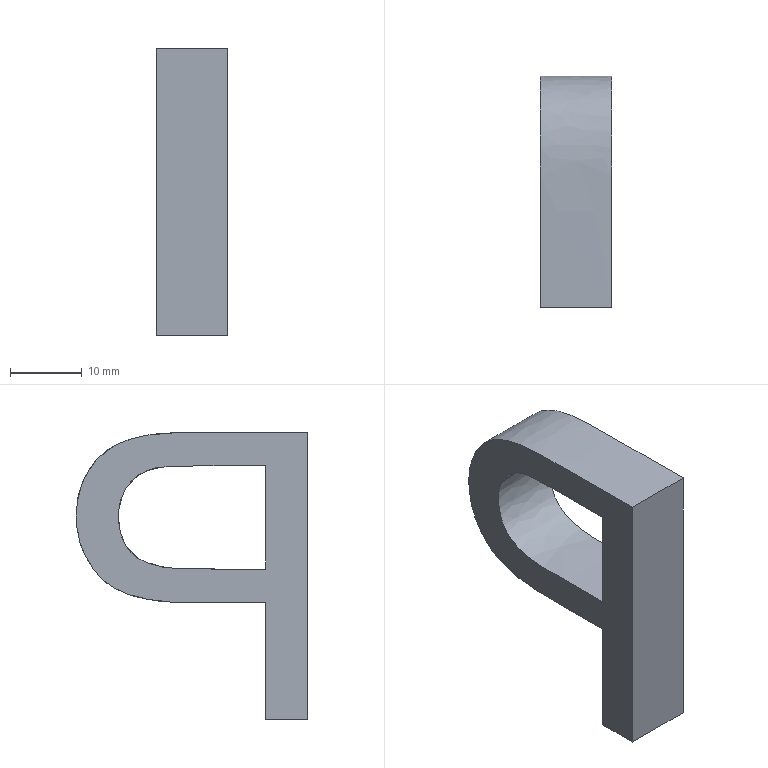Part | NX | features solid 2 | 1 solid | 8 faces | box 10 x 32.199 x 40 mm | volume 5391 mm3 | plane 6 | spline 2
STEP:
#1=CARTESIAN_POINT('',(2250.,-473.557,-634.665));
#2=VERTEX_POINT('',#1);
#3=CARTESIAN_POINT('',(2250.,-473.557,-649.029));
#4=VERTEX_POINT('',#3);
#5=CARTESIAN_POINT('',(2250.,-473.557,-634.665));
#6=CARTESIAN_POINT('',(2250.,-473.557,-639.453));
#7=CARTESIAN_POINT('',(2250.,-473.557,-644.241));
#8=CARTESIAN_POINT('',(2250.,-473.557,-649.029));
#9=B_SPLINE_CURVE_WITH_KNOTS('',3,(#5,#6,#7,#8),.UNSPECIFIED.,.F.,.F.,(4,4),(0.,0.1858),.PIECEWISE_BEZIER_KNOTS.);
#10=EDGE_CURVE('',#2,#4,#9,.T.);
#11=ORIENTED_EDGE('',*,*,#10,.F.);
#12=CARTESIAN_POINT('',(2260.,-473.557,-634.665));
#13=VERTEX_POINT('',#12);
#14=CARTESIAN_POINT('',(2260.,-473.557,-634.665));
#15=DIRECTION('',(-1.,0.,0.));
#16=VECTOR('',#15,1000.);
#17=LINE('',#14,#16);
#18=EDGE_CURVE('',#2,#13,#17,.F.);
#19=ORIENTED_EDGE('',*,*,#18,.T.);
#20=CARTESIAN_POINT('',(2260.,-473.557,-649.029));
#21=VERTEX_POINT('',#20);
#22=CARTESIAN_POINT('',(2260.,-473.557,-634.665));
#23=CARTESIAN_POINT('',(2260.,-473.557,-639.453));
#24=CARTESIAN_POINT('',(2260.,-473.557,-644.241));
#25=CARTESIAN_POINT('',(2260.,-473.557,-649.029));
#26=B_SPLINE_CURVE_WITH_KNOTS('',3,(#22,#23,#24,#25),.UNSPECIFIED.,.F.,.F.,(4,4),(0.,0.1858),.PIECEWISE_BEZIER_KNOTS.);
#27=EDGE_CURVE('',#13,#21,#26,.T.);
#28=ORIENTED_EDGE('',*,*,#27,.T.);
#29=CARTESIAN_POINT('',(2260.,-473.557,-649.029));
#30=DIRECTION('',(-1.,0.,0.));
#31=VECTOR('',#30,1000.);
#32=LINE('',#29,#31);
#33=EDGE_CURVE('',#21,#4,#32,.T.);
#34=ORIENTED_EDGE('',*,*,#33,.T.);
#35=EDGE_LOOP('',(#11,#19,#28,#34));
#36=FACE_BOUND('',#35,.T.);
#37=CARTESIAN_POINT('',(2260.,-473.557,-634.665));
#38=DIRECTION('',(0.,1.,0.));
#39=DIRECTION('',(-1.,0.,0.));
#40=AXIS2_PLACEMENT_3D('',#37,#38,#39);
#41=PLANE('',#40);
#42=ADVANCED_FACE('',(#36),#41,.T.);
#43=CARTESIAN_POINT('',(2250.,-473.557,-670.));
#44=VERTEX_POINT('',#43);
#45=CARTESIAN_POINT('',(2250.,-479.4,-670.));
#46=VERTEX_POINT('',#45);
#47=CARTESIAN_POINT('',(2250.,-473.557,-670.));
#48=CARTESIAN_POINT('',(2250.,-475.505,-670.));
#49=CARTESIAN_POINT('',(2250.,-477.452,-670.));
#50=CARTESIAN_POINT('',(2250.,-479.4,-670.));
#51=B_SPLINE_CURVE_WITH_KNOTS('',3,(#47,#48,#49,#50),.UNSPECIFIED.,.F.,.F.,(4,4),(0.,0.04053),.PIECEWISE_BEZIER_KNOTS.);
#52=EDGE_CURVE('',#44,#46,#51,.T.);
#53=ORIENTED_EDGE('',*,*,#52,.F.);
#54=CARTESIAN_POINT('',(2260.,-473.557,-670.));
#55=VERTEX_POINT('',#54);
#56=CARTESIAN_POINT('',(2260.,-473.557,-670.));
#57=DIRECTION('',(-1.,0.,0.));
#58=VECTOR('',#57,1000.);
#59=LINE('',#56,#58);
#60=EDGE_CURVE('',#55,#44,#59,.T.);
#61=ORIENTED_EDGE('',*,*,#60,.F.);
#62=CARTESIAN_POINT('',(2260.,-479.4,-670.));
#63=VERTEX_POINT('',#62);
#64=CARTESIAN_POINT('',(2260.,-473.557,-670.));
#65=CARTESIAN_POINT('',(2260.,-475.505,-670.));
#66=CARTESIAN_POINT('',(2260.,-477.452,-670.));
#67=CARTESIAN_POINT('',(2260.,-479.4,-670.));
#68=B_SPLINE_CURVE_WITH_KNOTS('',3,(#64,#65,#66,#67),.UNSPECIFIED.,.F.,.F.,(4,4),(0.,0.04053),.PIECEWISE_BEZIER_KNOTS.);
#69=EDGE_CURVE('',#55,#63,#68,.T.);
#70=ORIENTED_EDGE('',*,*,#69,.T.);
#71=CARTESIAN_POINT('',(2260.,-479.4,-670.));
#72=DIRECTION('',(-1.,0.,0.));
#73=VECTOR('',#72,1000.);
#74=LINE('',#71,#73);
#75=EDGE_CURVE('',#63,#46,#74,.T.);
#76=ORIENTED_EDGE('',*,*,#75,.T.);
#77=EDGE_LOOP('',(#53,#61,#70,#76));
#78=FACE_BOUND('',#77,.T.);
#79=CARTESIAN_POINT('',(2260.,-473.557,-670.));
#80=DIRECTION('',(0.,0.,-1.));
#81=DIRECTION('',(-1.,0.,0.));
#82=AXIS2_PLACEMENT_3D('',#79,#80,#81);
#83=PLANE('',#82);
#84=ADVANCED_FACE('',(#78),#83,.T.);
#85=CARTESIAN_POINT('',(2250.,-479.4,-630.));
#86=VERTEX_POINT('',#85);
#87=CARTESIAN_POINT('',(2250.,-479.4,-670.));
#88=CARTESIAN_POINT('',(2250.,-479.4,-656.667));
#89=CARTESIAN_POINT('',(2250.,-479.4,-643.333));
#90=CARTESIAN_POINT('',(2250.,-479.4,-630.));
#91=B_SPLINE_CURVE_WITH_KNOTS('',3,(#87,#88,#89,#90),.UNSPECIFIED.,.F.,.F.,(4,4),(0.04053,0.3179),.PIECEWISE_BEZIER_KNOTS.);
#92=EDGE_CURVE('',#46,#86,#91,.T.);
#93=ORIENTED_EDGE('',*,*,#92,.F.);
#94=ORIENTED_EDGE('',*,*,#75,.F.);
#95=CARTESIAN_POINT('',(2260.,-479.4,-630.));
#96=VERTEX_POINT('',#95);
#97=CARTESIAN_POINT('',(2260.,-479.4,-670.));
#98=CARTESIAN_POINT('',(2260.,-479.4,-656.667));
#99=CARTESIAN_POINT('',(2260.,-479.4,-643.333));
#100=CARTESIAN_POINT('',(2260.,-479.4,-630.));
#101=B_SPLINE_CURVE_WITH_KNOTS('',3,(#97,#98,#99,#100),.UNSPECIFIED.,.F.,.F.,(4,4),(0.04053,0.3179),.PIECEWISE_BEZIER_KNOTS.);
#102=EDGE_CURVE('',#63,#96,#101,.T.);
#103=ORIENTED_EDGE('',*,*,#102,.T.);
#104=CARTESIAN_POINT('',(2260.,-479.4,-630.));
#105=DIRECTION('',(-1.,0.,0.));
#106=VECTOR('',#105,1000.);
#107=LINE('',#104,#106);
#108=EDGE_CURVE('',#96,#86,#107,.T.);
#109=ORIENTED_EDGE('',*,*,#108,.T.);
#110=EDGE_LOOP('',(#93,#94,#103,#109));
#111=FACE_BOUND('',#110,.T.);
#112=CARTESIAN_POINT('',(2260.,-479.4,-670.));
#113=DIRECTION('',(0.,-1.,0.));
#114=DIRECTION('',(1.,0.,0.));
#115=AXIS2_PLACEMENT_3D('',#112,#113,#114);
#116=PLANE('',#115);
#117=ADVANCED_FACE('',(#111),#116,.T.);
#118=CARTESIAN_POINT('',(2250.,-473.557,-653.694));
#119=VERTEX_POINT('',#118);
#120=CARTESIAN_POINT('',(2250.,-479.4,-630.));
#121=CARTESIAN_POINT('',(2250.,-474.102,-630.));
#122=CARTESIAN_POINT('',(2250.,-468.805,-630.));
#123=CARTESIAN_POINT('',(2250.,-463.507,-630.02));
#124=CARTESIAN_POINT('',(2250.,-460.693,-630.031));
#125=CARTESIAN_POINT('',(2250.,-458.551,-630.153));
#126=CARTESIAN_POINT('',(2250.,-454.989,-630.747));
#127=CARTESIAN_POINT('',(2250.,-453.259,-631.361));
#128=CARTESIAN_POINT('',(2250.,-450.437,-633.202));
#129=CARTESIAN_POINT('',(2250.,-449.312,-634.497));
#130=CARTESIAN_POINT('',(2250.,-448.468,-636.14));
#131=CARTESIAN_POINT('',(2250.,-447.614,-637.801));
#132=CARTESIAN_POINT('',(2250.,-447.201,-639.621));
#133=CARTESIAN_POINT('',(2250.,-447.201,-644.975));
#134=CARTESIAN_POINT('',(2250.,-448.318,-647.866));
#135=CARTESIAN_POINT('',(2250.,-450.581,-650.206));
#136=CARTESIAN_POINT('',(2250.,-452.846,-652.547));
#137=CARTESIAN_POINT('',(2250.,-456.945,-653.725));
#138=CARTESIAN_POINT('',(2250.,-466.429,-653.676));
#139=CARTESIAN_POINT('',(2250.,-469.993,-653.694));
#140=CARTESIAN_POINT('',(2250.,-473.557,-653.694));
#141=B_SPLINE_CURVE_WITH_KNOTS('',3,(#120,#121,#122,#123,#124,#125,#126,#127,#128,#129,#130,#131,#132,#133,#134,#135,#136,#137,#138,#139,#140),.UNSPECIFIED.,.F.,.F.,(4,3,2,2,3,2,3,2,4),(0.3179,0.4282,0.4729,0.5366,0.6006,0.6433,0.7184,0.8183,0.8785),.UNSPECIFIED.);
#142=EDGE_CURVE('',#86,#119,#141,.T.);
#143=ORIENTED_EDGE('',*,*,#142,.F.);
#144=ORIENTED_EDGE('',*,*,#108,.F.);
#145=CARTESIAN_POINT('',(2260.,-473.557,-653.694));
#146=VERTEX_POINT('',#145);
#147=CARTESIAN_POINT('',(2260.,-479.4,-630.));
#148=CARTESIAN_POINT('',(2260.,-474.102,-630.));
#149=CARTESIAN_POINT('',(2260.,-468.805,-630.));
#150=CARTESIAN_POINT('',(2260.,-463.507,-630.02));
#151=CARTESIAN_POINT('',(2260.,-460.693,-630.031));
#152=CARTESIAN_POINT('',(2260.,-458.551,-630.153));
#153=CARTESIAN_POINT('',(2260.,-454.989,-630.747));
#154=CARTESIAN_POINT('',(2260.,-453.259,-631.361));
#155=CARTESIAN_POINT('',(2260.,-450.437,-633.202));
#156=CARTESIAN_POINT('',(2260.,-449.312,-634.497));
#157=CARTESIAN_POINT('',(2260.,-448.468,-636.14));
#158=CARTESIAN_POINT('',(2260.,-447.614,-637.801));
#159=CARTESIAN_POINT('',(2260.,-447.201,-639.621));
#160=CARTESIAN_POINT('',(2260.,-447.201,-644.975));
#161=CARTESIAN_POINT('',(2260.,-448.318,-647.866));
#162=CARTESIAN_POINT('',(2260.,-450.581,-650.206));
#163=CARTESIAN_POINT('',(2260.,-452.846,-652.547));
#164=CARTESIAN_POINT('',(2260.,-456.945,-653.725));
#165=CARTESIAN_POINT('',(2260.,-466.429,-653.676));
#166=CARTESIAN_POINT('',(2260.,-469.993,-653.694));
#167=CARTESIAN_POINT('',(2260.,-473.557,-653.694));
#168=B_SPLINE_CURVE_WITH_KNOTS('',3,(#147,#148,#149,#150,#151,#152,#153,#154,#155,#156,#157,#158,#159,#160,#161,#162,#163,#164,#165,#166,#167),.UNSPECIFIED.,.F.,.F.,(4,3,2,2,3,2,3,2,4),(0.3179,0.4282,0.4729,0.5366,0.6006,0.6433,0.7184,0.8183,0.8785),.UNSPECIFIED.);
#169=EDGE_CURVE('',#96,#146,#168,.T.);
#170=ORIENTED_EDGE('',*,*,#169,.T.);
#171=CARTESIAN_POINT('',(2260.,-473.557,-653.694));
#172=DIRECTION('',(-1.,0.,0.));
#173=VECTOR('',#172,1000.);
#174=LINE('',#171,#173);
#175=EDGE_CURVE('',#146,#119,#174,.T.);
#176=ORIENTED_EDGE('',*,*,#175,.T.);
#177=EDGE_LOOP('',(#143,#144,#170,#176));
#178=FACE_BOUND('',#177,.T.);
#179=CARTESIAN_POINT('',(2260.,-479.4,-630.));
#180=CARTESIAN_POINT('',(2250.,-479.4,-630.));
#181=CARTESIAN_POINT('',(2260.,-477.716,-630.));
#182=CARTESIAN_POINT('',(2250.,-477.716,-630.));
#183=CARTESIAN_POINT('',(2260.,-474.347,-630.));
#184=CARTESIAN_POINT('',(2250.,-474.347,-630.));
#185=CARTESIAN_POINT('',(2260.,-470.142,-630.003));
#186=CARTESIAN_POINT('',(2250.,-470.142,-630.003));
#187=CARTESIAN_POINT('',(2260.,-467.188,-630.009));
#188=CARTESIAN_POINT('',(2250.,-467.188,-630.009));
#189=CARTESIAN_POINT('',(2260.,-465.516,-630.013));
#190=CARTESIAN_POINT('',(2250.,-465.516,-630.013));
#191=CARTESIAN_POINT('',(2260.,-464.432,-630.017));
#192=CARTESIAN_POINT('',(2250.,-464.432,-630.017));
#193=CARTESIAN_POINT('',(2260.,-463.656,-630.019));
#194=CARTESIAN_POINT('',(2250.,-463.656,-630.019));
#195=CARTESIAN_POINT('',(2260.,-462.547,-630.025));
#196=CARTESIAN_POINT('',(2250.,-462.547,-630.025));
#197=CARTESIAN_POINT('',(2260.,-460.797,-630.061));
#198=CARTESIAN_POINT('',(2250.,-460.797,-630.061));
#199=CARTESIAN_POINT('',(2260.,-458.64,-630.177));
#200=CARTESIAN_POINT('',(2250.,-458.64,-630.177));
#201=CARTESIAN_POINT('',(2260.,-456.768,-630.425));
#202=CARTESIAN_POINT('',(2250.,-456.768,-630.425));
#203=CARTESIAN_POINT('',(2260.,-454.638,-630.914));
#204=CARTESIAN_POINT('',(2250.,-454.638,-630.914));
#205=CARTESIAN_POINT('',(2260.,-452.784,-631.656));
#206=CARTESIAN_POINT('',(2250.,-452.784,-631.656));
#207=CARTESIAN_POINT('',(2260.,-451.243,-632.668));
#208=CARTESIAN_POINT('',(2250.,-451.243,-632.668));
#209=CARTESIAN_POINT('',(2260.,-450.215,-633.593));
#210=CARTESIAN_POINT('',(2250.,-450.215,-633.593));
#211=CARTESIAN_POINT('',(2260.,-449.461,-634.509));
#212=CARTESIAN_POINT('',(2250.,-449.461,-634.509));
#213=CARTESIAN_POINT('',(2260.,-448.932,-635.3));
#214=CARTESIAN_POINT('',(2250.,-448.932,-635.3));
#215=CARTESIAN_POINT('',(2260.,-448.636,-635.819));
#216=CARTESIAN_POINT('',(2250.,-448.636,-635.819));
#217=CARTESIAN_POINT('',(2260.,-448.485,-636.106));
#218=CARTESIAN_POINT('',(2250.,-448.485,-636.106));
#219=CARTESIAN_POINT('',(2260.,-448.301,-636.471));
#220=CARTESIAN_POINT('',(2250.,-448.301,-636.471));
#221=CARTESIAN_POINT('',(2260.,-448.034,-637.063));
#222=CARTESIAN_POINT('',(2250.,-448.034,-637.063));
#223=CARTESIAN_POINT('',(2260.,-447.574,-638.322));
#224=CARTESIAN_POINT('',(2250.,-447.574,-638.322));
#225=CARTESIAN_POINT('',(2260.,-447.2,-640.182));
#226=CARTESIAN_POINT('',(2250.,-447.2,-640.182));
#227=CARTESIAN_POINT('',(2260.,-447.173,-642.595));
#228=CARTESIAN_POINT('',(2250.,-447.173,-642.595));
#229=CARTESIAN_POINT('',(2260.,-447.512,-644.822));
#230=CARTESIAN_POINT('',(2250.,-447.512,-644.822));
#231=CARTESIAN_POINT('',(2260.,-448.216,-646.878));
#232=CARTESIAN_POINT('',(2250.,-448.216,-646.878));
#233=CARTESIAN_POINT('',(2260.,-449.12,-648.452));
#234=CARTESIAN_POINT('',(2250.,-449.12,-648.452));
#235=CARTESIAN_POINT('',(2260.,-449.899,-649.459));
#236=CARTESIAN_POINT('',(2250.,-449.899,-649.459));
#237=CARTESIAN_POINT('',(2260.,-450.418,-650.04));
#238=CARTESIAN_POINT('',(2250.,-450.418,-650.04));
#239=CARTESIAN_POINT('',(2260.,-450.865,-650.499));
#240=CARTESIAN_POINT('',(2250.,-450.865,-650.499));
#241=CARTESIAN_POINT('',(2260.,-451.392,-650.953));
#242=CARTESIAN_POINT('',(2250.,-451.392,-650.953));
#243=CARTESIAN_POINT('',(2260.,-452.396,-651.655));
#244=CARTESIAN_POINT('',(2250.,-452.396,-651.655));
#245=CARTESIAN_POINT('',(2260.,-453.845,-652.382));
#246=CARTESIAN_POINT('',(2250.,-453.845,-652.382));
#247=CARTESIAN_POINT('',(2260.,-456.626,-653.262));
#248=CARTESIAN_POINT('',(2250.,-456.626,-653.262));
#249=CARTESIAN_POINT('',(2260.,-460.057,-653.716));
#250=CARTESIAN_POINT('',(2250.,-460.057,-653.716));
#251=CARTESIAN_POINT('',(2260.,-464.22,-653.685));
#252=CARTESIAN_POINT('',(2250.,-464.22,-653.685));
#253=CARTESIAN_POINT('',(2260.,-468.367,-653.686));
#254=CARTESIAN_POINT('',(2250.,-468.367,-653.686));
#255=CARTESIAN_POINT('',(2260.,-471.482,-653.694));
#256=CARTESIAN_POINT('',(2250.,-471.482,-653.694));
#257=CARTESIAN_POINT('',(2260.,-473.557,-653.694));
#258=CARTESIAN_POINT('',(2250.,-473.557,-653.694));
#259=B_SPLINE_SURFACE_WITH_KNOTS('',3,1,((#179,#180),(#181,#182),(#183,#184),(#185,#186),(#187,#188),(#189,#190),(#191,#192),(#193,#194),(#195,#196),(#197,#198),(#199,#200),(#201,#202),(#203,#204),(#205,#206),(#207,#208),(#209,#210),(#211,#212),(#213,#214),(#215,#216),(#217,#218),(#219,#220),(#221,#222),(#223,#224),(#225,#226),(#227,#228),(#229,#230),(#231,#232),(#233,#234),(#235,#236),(#237,#238),(#239,#240),(#241,#242),(#243,#244),(#245,#246),(#247,#248),(#249,#250),(#251,#252),(#253,#254),(#255,#256),(#257,#258)),.SURF_OF_LINEAR_EXTRUSION.,.F.,.F.,.F.,(4,1,1,1,1,1,1,1,1,1,1,1,1,1,1,1,1,1,1,1,1,1,1,1,1,1,1,1,1,1,1,1,1,1,1,1,1,4),(2,2),(0.3179,0.353,0.388,0.4055,0.4143,0.423,0.4274,0.4318,0.4406,0.4581,0.4756,0.4931,0.5282,0.5457,0.5632,0.5807,0.5895,0.5982,0.6004,0.6026,0.607,0.6157,0.6333,0.6508,0.6683,0.6858,0.7033,0.7121,0.7165,0.7208,0.7296,0.7384,0.7559,0.7734,0.8084,0.8259,0.8435,0.8785),(0.,1.),.UNSPECIFIED.);
#260=ADVANCED_FACE('',(#178),#259,.T.);
#261=CARTESIAN_POINT('',(2250.,-473.557,-653.694));
#262=CARTESIAN_POINT('',(2250.,-473.557,-659.129));
#263=CARTESIAN_POINT('',(2250.,-473.557,-664.565));
#264=CARTESIAN_POINT('',(2250.,-473.557,-670.));
#265=B_SPLINE_CURVE_WITH_KNOTS('',3,(#261,#262,#263,#264),.UNSPECIFIED.,.F.,.F.,(4,4),(0.8785,1.),.PIECEWISE_BEZIER_KNOTS.);
#266=EDGE_CURVE('',#119,#44,#265,.T.);
#267=ORIENTED_EDGE('',*,*,#266,.F.);
#268=ORIENTED_EDGE('',*,*,#175,.F.);
#269=CARTESIAN_POINT('',(2260.,-473.557,-653.694));
#270=CARTESIAN_POINT('',(2260.,-473.557,-659.129));
#271=CARTESIAN_POINT('',(2260.,-473.557,-664.565));
#272=CARTESIAN_POINT('',(2260.,-473.557,-670.));
#273=B_SPLINE_CURVE_WITH_KNOTS('',3,(#269,#270,#271,#272),.UNSPECIFIED.,.F.,.F.,(4,4),(0.8785,1.),.PIECEWISE_BEZIER_KNOTS.);
#274=EDGE_CURVE('',#146,#55,#273,.T.);
#275=ORIENTED_EDGE('',*,*,#274,.T.);
#276=ORIENTED_EDGE('',*,*,#60,.T.);
#277=EDGE_LOOP('',(#267,#268,#275,#276));
#278=FACE_BOUND('',#277,.T.);
#279=CARTESIAN_POINT('',(2260.,-473.557,-653.694));
#280=DIRECTION('',(0.,1.,0.));
#281=DIRECTION('',(-1.,0.,0.));
#282=AXIS2_PLACEMENT_3D('',#279,#280,#281);
#283=PLANE('',#282);
#284=ADVANCED_FACE('',(#278),#283,.T.);
#285=CARTESIAN_POINT('',(2250.,-473.557,-649.029));
#286=CARTESIAN_POINT('',(2250.,-469.993,-649.029));
#287=CARTESIAN_POINT('',(2250.,-466.429,-649.029));
#288=CARTESIAN_POINT('',(2250.,-459.3,-649.029));
#289=CARTESIAN_POINT('',(2250.,-456.761,-648.432));
#290=CARTESIAN_POINT('',(2250.,-453.801,-645.869));
#291=CARTESIAN_POINT('',(2250.,-453.06,-644.057));
#292=CARTESIAN_POINT('',(2250.,-453.06,-640.08));
#293=CARTESIAN_POINT('',(2250.,-453.473,-638.642));
#294=CARTESIAN_POINT('',(2250.,-455.24,-636.236));
#295=CARTESIAN_POINT('',(2250.,-456.394,-635.446));
#296=CARTESIAN_POINT('',(2250.,-457.837,-635.052));
#297=CARTESIAN_POINT('',(2250.,-458.75,-634.803));
#298=CARTESIAN_POINT('',(2250.,-460.448,-634.681));
#299=CARTESIAN_POINT('',(2250.,-466.49,-634.644));
#300=CARTESIAN_POINT('',(2250.,-470.023,-634.665));
#301=CARTESIAN_POINT('',(2250.,-473.557,-634.665));
#302=B_SPLINE_CURVE_WITH_KNOTS('',3,(#285,#286,#287,#288,#289,#290,#291,#292,#293,#294,#295,#296,#297,#298,#299,#300,#301),.UNSPECIFIED.,.F.,.F.,(4,2,2,2,2,3,2,4),(0.1858,0.324,0.4623,0.5999,0.6976,0.7946,0.8799,1.),.UNSPECIFIED.);
#303=EDGE_CURVE('',#4,#2,#302,.T.);
#304=ORIENTED_EDGE('',*,*,#303,.F.);
#305=ORIENTED_EDGE('',*,*,#33,.F.);
#306=CARTESIAN_POINT('',(2260.,-473.557,-649.029));
#307=CARTESIAN_POINT('',(2260.,-469.993,-649.029));
#308=CARTESIAN_POINT('',(2260.,-466.429,-649.029));
#309=CARTESIAN_POINT('',(2260.,-459.3,-649.029));
#310=CARTESIAN_POINT('',(2260.,-456.761,-648.432));
#311=CARTESIAN_POINT('',(2260.,-453.801,-645.869));
#312=CARTESIAN_POINT('',(2260.,-453.06,-644.057));
#313=CARTESIAN_POINT('',(2260.,-453.06,-640.08));
#314=CARTESIAN_POINT('',(2260.,-453.473,-638.642));
#315=CARTESIAN_POINT('',(2260.,-455.24,-636.236));
#316=CARTESIAN_POINT('',(2260.,-456.394,-635.446));
#317=CARTESIAN_POINT('',(2260.,-457.837,-635.052));
#318=CARTESIAN_POINT('',(2260.,-458.75,-634.803));
#319=CARTESIAN_POINT('',(2260.,-460.448,-634.681));
#320=CARTESIAN_POINT('',(2260.,-466.49,-634.644));
#321=CARTESIAN_POINT('',(2260.,-470.023,-634.665));
#322=CARTESIAN_POINT('',(2260.,-473.557,-634.665));
#323=B_SPLINE_CURVE_WITH_KNOTS('',3,(#306,#307,#308,#309,#310,#311,#312,#313,#314,#315,#316,#317,#318,#319,#320,#321,#322),.UNSPECIFIED.,.F.,.F.,(4,2,2,2,2,3,2,4),(0.1858,0.324,0.4623,0.5999,0.6976,0.7946,0.8799,1.),.UNSPECIFIED.);
#324=EDGE_CURVE('',#21,#13,#323,.T.);
#325=ORIENTED_EDGE('',*,*,#324,.T.);
#326=ORIENTED_EDGE('',*,*,#18,.F.);
#327=EDGE_LOOP('',(#304,#305,#325,#326));
#328=FACE_BOUND('',#327,.T.);
#329=CARTESIAN_POINT('',(2260.,-473.557,-649.029));
#330=CARTESIAN_POINT('',(2250.,-473.557,-649.029));
#331=CARTESIAN_POINT('',(2260.,-470.933,-649.029));
#332=CARTESIAN_POINT('',(2250.,-470.933,-649.029));
#333=CARTESIAN_POINT('',(2260.,-467.653,-649.03));
#334=CARTESIAN_POINT('',(2250.,-467.653,-649.03));
#335=CARTESIAN_POINT('',(2260.,-463.72,-649.028));
#336=CARTESIAN_POINT('',(2250.,-463.72,-649.028));
#337=CARTESIAN_POINT('',(2260.,-461.089,-649.033));
#338=CARTESIAN_POINT('',(2250.,-461.089,-649.033));
#339=CARTESIAN_POINT('',(2260.,-458.368,-648.704));
#340=CARTESIAN_POINT('',(2250.,-458.368,-648.704));
#341=CARTESIAN_POINT('',(2260.,-455.925,-647.805));
#342=CARTESIAN_POINT('',(2250.,-455.925,-647.805));
#343=CARTESIAN_POINT('',(2260.,-454.352,-646.342));
#344=CARTESIAN_POINT('',(2250.,-454.352,-646.342));
#345=CARTESIAN_POINT('',(2260.,-453.351,-644.476));
#346=CARTESIAN_POINT('',(2250.,-453.351,-644.476));
#347=CARTESIAN_POINT('',(2260.,-452.963,-642.117));
#348=CARTESIAN_POINT('',(2250.,-452.963,-642.117));
#349=CARTESIAN_POINT('',(2260.,-453.189,-639.561));
#350=CARTESIAN_POINT('',(2250.,-453.189,-639.561));
#351=CARTESIAN_POINT('',(2260.,-454.169,-637.471));
#352=CARTESIAN_POINT('',(2250.,-454.169,-637.471));
#353=CARTESIAN_POINT('',(2260.,-455.539,-636.102));
#354=CARTESIAN_POINT('',(2250.,-455.539,-636.102));
#355=CARTESIAN_POINT('',(2260.,-456.797,-635.388));
#356=CARTESIAN_POINT('',(2250.,-456.797,-635.388));
#357=CARTESIAN_POINT('',(2260.,-457.77,-635.053));
#358=CARTESIAN_POINT('',(2250.,-457.77,-635.053));
#359=CARTESIAN_POINT('',(2260.,-458.347,-634.935));
#360=CARTESIAN_POINT('',(2250.,-458.347,-634.935));
#361=CARTESIAN_POINT('',(2260.,-459.137,-634.819));
#362=CARTESIAN_POINT('',(2250.,-459.137,-634.819));
#363=CARTESIAN_POINT('',(2260.,-460.361,-634.721));
#364=CARTESIAN_POINT('',(2250.,-460.361,-634.721));
#365=CARTESIAN_POINT('',(2260.,-462.283,-634.663));
#366=CARTESIAN_POINT('',(2250.,-462.283,-634.663));
#367=CARTESIAN_POINT('',(2260.,-465.35,-634.656));
#368=CARTESIAN_POINT('',(2250.,-465.35,-634.656));
#369=CARTESIAN_POINT('',(2260.,-469.056,-634.657));
#370=CARTESIAN_POINT('',(2250.,-469.056,-634.657));
#371=CARTESIAN_POINT('',(2260.,-472.06,-634.665));
#372=CARTESIAN_POINT('',(2250.,-472.06,-634.665));
#373=CARTESIAN_POINT('',(2260.,-473.557,-634.665));
#374=CARTESIAN_POINT('',(2250.,-473.557,-634.665));
#375=B_SPLINE_SURFACE_WITH_KNOTS('',3,1,((#329,#330),(#331,#332),(#333,#334),(#335,#336),(#337,#338),(#339,#340),(#341,#342),(#343,#344),(#345,#346),(#347,#348),(#349,#350),(#351,#352),(#353,#354),(#355,#356),(#357,#358),(#359,#360),(#361,#362),(#363,#364),(#365,#366),(#367,#368),(#369,#370),(#371,#372),(#373,#374)),.SURF_OF_LINEAR_EXTRUSION.,.F.,.F.,.F.,(4,1,1,1,1,1,1,1,1,1,1,1,1,1,1,1,1,1,1,1,4),(2,2),(0.1858,0.2875,0.313,0.3384,0.3893,0.4402,0.4911,0.542,0.5929,0.6438,0.6947,0.7455,0.771,0.7964,0.8092,0.8219,0.8473,0.8728,0.8982,0.9491,1.),(0.,1.),.UNSPECIFIED.);
#376=ADVANCED_FACE('',(#328),#375,.T.);
#377=ORIENTED_EDGE('',*,*,#69,.F.);
#378=ORIENTED_EDGE('',*,*,#274,.F.);
#379=ORIENTED_EDGE('',*,*,#169,.F.);
#380=ORIENTED_EDGE('',*,*,#102,.F.);
#381=EDGE_LOOP('',(#377,#378,#379,#380));
#382=FACE_BOUND('',#381,.T.);
#383=ORIENTED_EDGE('',*,*,#27,.F.);
#384=ORIENTED_EDGE('',*,*,#324,.F.);
#385=EDGE_LOOP('',(#383,#384));
#386=FACE_BOUND('',#385,.T.);
#387=CARTESIAN_POINT('',(2260.,-448.562,-635.96));
#388=DIRECTION('',(1.,0.,0.));
#389=DIRECTION('',(0.,1.,0.));
#390=AXIS2_PLACEMENT_3D('',#387,#388,#389);
#391=PLANE('',#390);
#392=ADVANCED_FACE('',(#382,#386),#391,.T.);
#393=ORIENTED_EDGE('',*,*,#52,.T.);
#394=ORIENTED_EDGE('',*,*,#92,.T.);
#395=ORIENTED_EDGE('',*,*,#142,.T.);
#396=ORIENTED_EDGE('',*,*,#266,.T.);
#397=EDGE_LOOP('',(#393,#394,#395,#396));
#398=FACE_BOUND('',#397,.T.);
#399=ORIENTED_EDGE('',*,*,#10,.T.);
#400=ORIENTED_EDGE('',*,*,#303,.T.);
#401=EDGE_LOOP('',(#399,#400));
#402=FACE_BOUND('',#401,.T.);
#403=CARTESIAN_POINT('',(2250.,-448.562,-635.96));
#404=DIRECTION('',(1.,0.,0.));
#405=DIRECTION('',(0.,1.,0.));
#406=AXIS2_PLACEMENT_3D('',#403,#404,#405);
#407=PLANE('',#406);
#408=ADVANCED_FACE('',(#398,#402),#407,.F.);
#409=CLOSED_SHELL('',(#42,#84,#117,#260,#284,#376,#392,#408));
#410=MANIFOLD_SOLID_BREP('',#409);
#411=(LENGTH_UNIT()NAMED_UNIT(*)SI_UNIT(.MILLI.,.METRE.));
#412=UNCERTAINTY_MEASURE_WITH_UNIT(LENGTH_MEASURE(0.0508),#411,'','');
#413=(NAMED_UNIT(*)PLANE_ANGLE_UNIT()SI_UNIT($,.RADIAN.));
#414=(NAMED_UNIT(*)SI_UNIT($,.STERADIAN.)SOLID_ANGLE_UNIT());
#415=(GEOMETRIC_REPRESENTATION_CONTEXT(3)GLOBAL_UNCERTAINTY_ASSIGNED_CONTEXT((#412))GLOBAL_UNIT_ASSIGNED_CONTEXT((#411,#413,#414))REPRESENTATION_CONTEXT('',''));
#416=ADVANCED_BREP_SHAPE_REPRESENTATION('',(#410),#415);